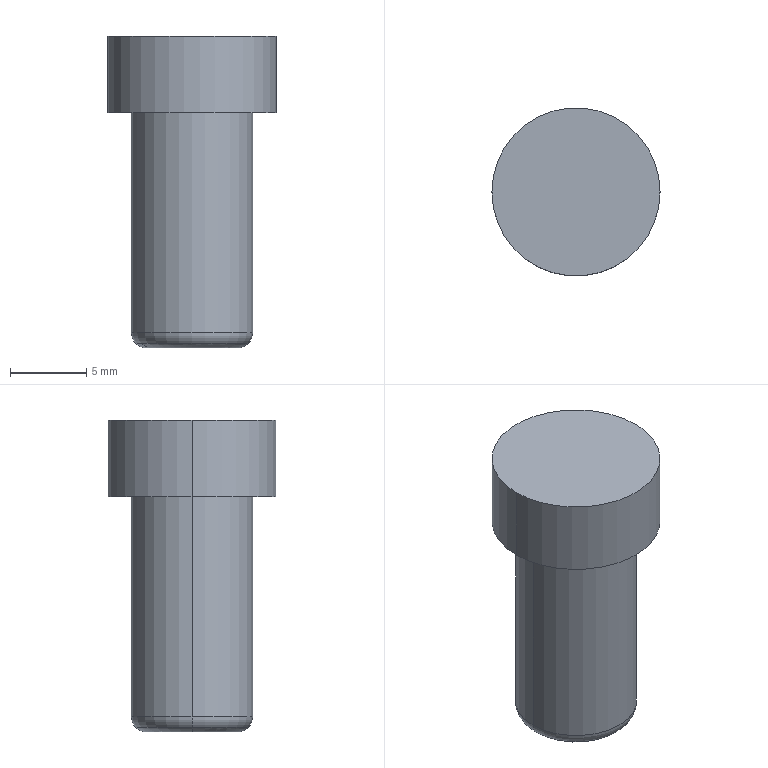Part | STEP file | 1_id1490_x_t | 1 solid | 11 faces | box 11 x 11 x 20.4 mm | volume 1232 mm3 | cylinder 4 | torus 4 | plane 3 | commonest cylinder face diameters 7.938 x2 11 x2
STEP:
#1=CARTESIAN_POINT('',(0.,0.,0.));
#2=DIRECTION('',(0.,0.,1.));
#3=DIRECTION('',(1.,0.,0.));
#4=AXIS2_PLACEMENT_3D('',#1,#2,#3);
#5=CARTESIAN_POINT('',(199.65,177.5,23.335));
#6=VERTEX_POINT('',#5);
#7=CARTESIAN_POINT('',(199.65,177.5,18.335));
#8=VERTEX_POINT('',#7);
#9=CARTESIAN_POINT('',(199.65,177.5,23.335));
#10=DIRECTION('',(0.,0.,-1.));
#11=VECTOR('',#10,1.);
#12=LINE('',#9,#11);
#13=CARTESIAN_POINT('',(194.15,177.5,23.335));
#14=DIRECTION('',(0.,0.,-1.));
#15=DIRECTION('',(-1.,0.,0.));
#16=AXIS2_PLACEMENT_3D('',#13,#14,#15);
#17=CYLINDRICAL_SURFACE('',#16,5.5);
#18=CARTESIAN_POINT('',(3.142,0.));
#19=DIRECTION('',(0.,1.));
#20=VECTOR('',#19,1.);
#21=LINE('',#18,#20);
#22=(GEOMETRIC_REPRESENTATION_CONTEXT(2)PARAMETRIC_REPRESENTATION_CONTEXT()REPRESENTATION_CONTEXT('',''));
#23=DEFINITIONAL_REPRESENTATION('',(#21),#22);
#24=PCURVE('',#17,#23);
#25=CARTESIAN_POINT('',(194.15,177.5,23.335));
#26=DIRECTION('',(0.,0.,-1.));
#27=DIRECTION('',(-1.,0.,0.));
#28=AXIS2_PLACEMENT_3D('',#25,#26,#27);
#29=CYLINDRICAL_SURFACE('',#28,5.5);
#30=CARTESIAN_POINT('',(3.142,0.));
#31=DIRECTION('',(0.,1.));
#32=VECTOR('',#31,1.);
#33=LINE('',#30,#32);
#34=(GEOMETRIC_REPRESENTATION_CONTEXT(2)PARAMETRIC_REPRESENTATION_CONTEXT()REPRESENTATION_CONTEXT('',''));
#35=DEFINITIONAL_REPRESENTATION('',(#33),#34);
#36=PCURVE('',#29,#35);
#37=SURFACE_CURVE('',#12,(#24,#36),.PCURVE_S1.);
#38=EDGE_CURVE('',#6,#8,#37,.T.);
#39=ORIENTED_EDGE('',*,*,#38,.F.);
#40=CARTESIAN_POINT('',(188.65,177.5,23.335));
#41=VERTEX_POINT('',#40);
#42=CARTESIAN_POINT('',(194.15,177.5,23.335));
#43=DIRECTION('',(0.,0.,1.));
#44=DIRECTION('',(-1.,0.,0.));
#45=AXIS2_PLACEMENT_3D('',#42,#43,#44);
#46=CIRCLE('',#45,5.5);
#47=CARTESIAN_POINT('',(6.283,0.));
#48=DIRECTION('',(-1.,0.));
#49=VECTOR('',#48,1.);
#50=LINE('',#47,#49);
#51=(GEOMETRIC_REPRESENTATION_CONTEXT(2)PARAMETRIC_REPRESENTATION_CONTEXT()REPRESENTATION_CONTEXT('',''));
#52=DEFINITIONAL_REPRESENTATION('',(#50),#51);
#53=PCURVE('',#17,#52);
#54=CARTESIAN_POINT('',(194.15,177.5,23.335));
#55=DIRECTION('',(0.,0.,1.));
#56=DIRECTION('',(1.,0.,0.));
#57=AXIS2_PLACEMENT_3D('',#54,#55,#56);
#58=PLANE('',#57);
#59=CARTESIAN_POINT('',(0.,0.));
#60=DIRECTION('',(-1.,0.));
#61=AXIS2_PLACEMENT_2D('',#59,#60);
#62=CIRCLE('',#61,5.5);
#63=(GEOMETRIC_REPRESENTATION_CONTEXT(2)PARAMETRIC_REPRESENTATION_CONTEXT()REPRESENTATION_CONTEXT('',''));
#64=DEFINITIONAL_REPRESENTATION('',(#62),#63);
#65=PCURVE('',#58,#64);
#66=SURFACE_CURVE('',#46,(#53,#65),.PCURVE_S1.);
#67=EDGE_CURVE('',#41,#6,#66,.T.);
#68=ORIENTED_EDGE('',*,*,#67,.F.);
#69=CARTESIAN_POINT('',(188.65,177.5,18.335));
#70=VERTEX_POINT('',#69);
#71=CARTESIAN_POINT('',(188.65,177.5,23.335));
#72=DIRECTION('',(0.,0.,1.));
#73=VECTOR('',#72,1.);
#74=LINE('',#71,#73);
#75=CARTESIAN_POINT('',(6.283,0.));
#76=DIRECTION('',(0.,-1.));
#77=VECTOR('',#76,1.);
#78=LINE('',#75,#77);
#79=(GEOMETRIC_REPRESENTATION_CONTEXT(2)PARAMETRIC_REPRESENTATION_CONTEXT()REPRESENTATION_CONTEXT('',''));
#80=DEFINITIONAL_REPRESENTATION('',(#78),#79);
#81=PCURVE('',#17,#80);
#82=CARTESIAN_POINT('',(0.,0.));
#83=DIRECTION('',(0.,-1.));
#84=VECTOR('',#83,1.);
#85=LINE('',#82,#84);
#86=(GEOMETRIC_REPRESENTATION_CONTEXT(2)PARAMETRIC_REPRESENTATION_CONTEXT()REPRESENTATION_CONTEXT('',''));
#87=DEFINITIONAL_REPRESENTATION('',(#85),#86);
#88=PCURVE('',#29,#87);
#89=SURFACE_CURVE('',#74,(#81,#88),.PCURVE_S1.);
#90=EDGE_CURVE('',#70,#41,#89,.T.);
#91=ORIENTED_EDGE('',*,*,#90,.F.);
#92=CARTESIAN_POINT('',(194.15,177.5,18.335));
#93=DIRECTION('',(0.,0.,-1.));
#94=DIRECTION('',(1.,0.,0.));
#95=AXIS2_PLACEMENT_3D('',#92,#93,#94);
#96=CIRCLE('',#95,5.5);
#97=CARTESIAN_POINT('',(3.142,5.));
#98=DIRECTION('',(1.,0.));
#99=VECTOR('',#98,1.);
#100=LINE('',#97,#99);
#101=(GEOMETRIC_REPRESENTATION_CONTEXT(2)PARAMETRIC_REPRESENTATION_CONTEXT()REPRESENTATION_CONTEXT('',''));
#102=DEFINITIONAL_REPRESENTATION('',(#100),#101);
#103=PCURVE('',#17,#102);
#104=CARTESIAN_POINT('',(194.15,177.5,18.335));
#105=DIRECTION('',(0.,0.,-1.));
#106=DIRECTION('',(-1.,0.,0.));
#107=AXIS2_PLACEMENT_3D('',#104,#105,#106);
#108=PLANE('',#107);
#109=CARTESIAN_POINT('',(0.,0.));
#110=DIRECTION('',(-1.,0.));
#111=AXIS2_PLACEMENT_2D('',#109,#110);
#112=CIRCLE('',#111,5.5);
#113=(GEOMETRIC_REPRESENTATION_CONTEXT(2)PARAMETRIC_REPRESENTATION_CONTEXT()REPRESENTATION_CONTEXT('',''));
#114=DEFINITIONAL_REPRESENTATION('',(#112),#113);
#115=PCURVE('',#108,#114);
#116=SURFACE_CURVE('',#96,(#103,#115),.PCURVE_S1.);
#117=EDGE_CURVE('',#8,#70,#116,.T.);
#118=ORIENTED_EDGE('',*,*,#117,.F.);
#119=EDGE_LOOP('',(#39,#68,#91,#118));
#120=FACE_BOUND('',#119,.T.);
#121=ADVANCED_FACE('',(#120),#17,.T.);
#122=ORIENTED_EDGE('',*,*,#117,.T.);
#123=CARTESIAN_POINT('',(194.15,177.5,18.335));
#124=DIRECTION('',(0.,0.,-1.));
#125=DIRECTION('',(-1.,0.,0.));
#126=AXIS2_PLACEMENT_3D('',#123,#124,#125);
#127=CIRCLE('',#126,5.5);
#128=CARTESIAN_POINT('',(0.,0.));
#129=DIRECTION('',(1.,0.));
#130=AXIS2_PLACEMENT_2D('',#128,#129);
#131=CIRCLE('',#130,5.5);
#132=(GEOMETRIC_REPRESENTATION_CONTEXT(2)PARAMETRIC_REPRESENTATION_CONTEXT()REPRESENTATION_CONTEXT('',''));
#133=DEFINITIONAL_REPRESENTATION('',(#131),#132);
#134=PCURVE('',#108,#133);
#135=CARTESIAN_POINT('',(0.,5.));
#136=DIRECTION('',(1.,0.));
#137=VECTOR('',#136,1.);
#138=LINE('',#135,#137);
#139=(GEOMETRIC_REPRESENTATION_CONTEXT(2)PARAMETRIC_REPRESENTATION_CONTEXT()REPRESENTATION_CONTEXT('',''));
#140=DEFINITIONAL_REPRESENTATION('',(#138),#139);
#141=PCURVE('',#29,#140);
#142=SURFACE_CURVE('',#127,(#134,#141),.PCURVE_S1.);
#143=EDGE_CURVE('',#70,#8,#142,.T.);
#144=ORIENTED_EDGE('',*,*,#143,.T.);
#145=EDGE_LOOP('',(#122,#144));
#146=FACE_BOUND('',#145,.T.);
#147=CARTESIAN_POINT('',(190.181,177.5,18.335));
#148=VERTEX_POINT('',#147);
#149=CARTESIAN_POINT('',(198.119,177.5,18.335));
#150=VERTEX_POINT('',#149);
#151=CARTESIAN_POINT('',(194.15,177.5,18.335));
#152=DIRECTION('',(0.,0.,1.));
#153=DIRECTION('',(-1.,0.,0.));
#154=AXIS2_PLACEMENT_3D('',#151,#152,#153);
#155=CIRCLE('',#154,3.969);
#156=CARTESIAN_POINT('',(3.969,0.));
#157=CARTESIAN_POINT('',(3.969,-6.874));
#158=CARTESIAN_POINT('',(-1.984,-3.437));
#159=CARTESIAN_POINT('',(-7.938,0.));
#160=CARTESIAN_POINT('',(-1.984,3.437));
#161=CARTESIAN_POINT('',(3.969,6.874));
#162=CARTESIAN_POINT('',(3.969,0.));
#163=(BOUNDED_CURVE()B_SPLINE_CURVE(2,(#156,#157,#158,#159,#160,#161,#162),.UNSPECIFIED.,.T.,.F.)B_SPLINE_CURVE_WITH_KNOTS((1,2,2,2,2,1),(-2.094,0.,2.094,4.189,6.283,8.378),.UNSPECIFIED.)CURVE()GEOMETRIC_REPRESENTATION_ITEM()RATIONAL_B_SPLINE_CURVE((1.,0.5,1.,0.5,1.,0.5,1.))REPRESENTATION_ITEM(''));
#164=(GEOMETRIC_REPRESENTATION_CONTEXT(2)PARAMETRIC_REPRESENTATION_CONTEXT()REPRESENTATION_CONTEXT('',''));
#165=DEFINITIONAL_REPRESENTATION('',(#163),#164);
#166=PCURVE('',#108,#165);
#167=CARTESIAN_POINT('',(194.15,177.5,23.335));
#168=DIRECTION('',(0.,0.,-1.));
#169=DIRECTION('',(-1.,0.,0.));
#170=AXIS2_PLACEMENT_3D('',#167,#168,#169);
#171=CYLINDRICAL_SURFACE('',#170,3.969);
#172=CARTESIAN_POINT('',(6.283,5.));
#173=DIRECTION('',(-1.,0.));
#174=VECTOR('',#173,1.);
#175=LINE('',#172,#174);
#176=(GEOMETRIC_REPRESENTATION_CONTEXT(2)PARAMETRIC_REPRESENTATION_CONTEXT()REPRESENTATION_CONTEXT('',''));
#177=DEFINITIONAL_REPRESENTATION('',(#175),#176);
#178=PCURVE('',#171,#177);
#179=SURFACE_CURVE('',#155,(#166,#178),.PCURVE_S1.);
#180=EDGE_CURVE('',#148,#150,#179,.T.);
#181=ORIENTED_EDGE('',*,*,#180,.T.);
#182=CARTESIAN_POINT('',(194.15,177.5,18.335));
#183=DIRECTION('',(0.,0.,1.));
#184=DIRECTION('',(1.,0.,0.));
#185=AXIS2_PLACEMENT_3D('',#182,#183,#184);
#186=CIRCLE('',#185,3.969);
#187=CARTESIAN_POINT('',(-3.969,0.));
#188=CARTESIAN_POINT('',(-3.969,6.874));
#189=CARTESIAN_POINT('',(1.984,3.437));
#190=CARTESIAN_POINT('',(7.938,0.));
#191=CARTESIAN_POINT('',(1.984,-3.437));
#192=CARTESIAN_POINT('',(-3.969,-6.874));
#193=CARTESIAN_POINT('',(-3.969,0.));
#194=(BOUNDED_CURVE()B_SPLINE_CURVE(2,(#187,#188,#189,#190,#191,#192,#193),.UNSPECIFIED.,.T.,.F.)B_SPLINE_CURVE_WITH_KNOTS((1,2,2,2,2,1),(-2.094,0.,2.094,4.189,6.283,8.378),.UNSPECIFIED.)CURVE()GEOMETRIC_REPRESENTATION_ITEM()RATIONAL_B_SPLINE_CURVE((1.,0.5,1.,0.5,1.,0.5,1.))REPRESENTATION_ITEM(''));
#195=(GEOMETRIC_REPRESENTATION_CONTEXT(2)PARAMETRIC_REPRESENTATION_CONTEXT()REPRESENTATION_CONTEXT('',''));
#196=DEFINITIONAL_REPRESENTATION('',(#194),#195);
#197=PCURVE('',#108,#196);
#198=CARTESIAN_POINT('',(194.15,177.5,23.335));
#199=DIRECTION('',(0.,0.,-1.));
#200=DIRECTION('',(-1.,0.,0.));
#201=AXIS2_PLACEMENT_3D('',#198,#199,#200);
#202=CYLINDRICAL_SURFACE('',#201,3.969);
#203=CARTESIAN_POINT('',(3.142,5.));
#204=DIRECTION('',(-1.,0.));
#205=VECTOR('',#204,1.);
#206=LINE('',#203,#205);
#207=(GEOMETRIC_REPRESENTATION_CONTEXT(2)PARAMETRIC_REPRESENTATION_CONTEXT()REPRESENTATION_CONTEXT('',''));
#208=DEFINITIONAL_REPRESENTATION('',(#206),#207);
#209=PCURVE('',#202,#208);
#210=SURFACE_CURVE('',#186,(#197,#209),.PCURVE_S1.);
#211=EDGE_CURVE('',#150,#148,#210,.T.);
#212=ORIENTED_EDGE('',*,*,#211,.T.);
#213=EDGE_LOOP('',(#181,#212));
#214=FACE_BOUND('',#213,.T.);
#215=ADVANCED_FACE('',(#146,#214),#108,.T.);
#216=CARTESIAN_POINT('',(198.119,177.5,3.935));
#217=VERTEX_POINT('',#216);
#218=CARTESIAN_POINT('',(198.119,177.5,18.335));
#219=DIRECTION('',(0.,0.,-1.));
#220=VECTOR('',#219,1.);
#221=LINE('',#218,#220);
#222=CARTESIAN_POINT('',(3.142,5.));
#223=DIRECTION('',(0.,1.));
#224=VECTOR('',#223,1.);
#225=LINE('',#222,#224);
#226=(GEOMETRIC_REPRESENTATION_CONTEXT(2)PARAMETRIC_REPRESENTATION_CONTEXT()REPRESENTATION_CONTEXT('',''));
#227=DEFINITIONAL_REPRESENTATION('',(#225),#226);
#228=PCURVE('',#202,#227);
#229=CARTESIAN_POINT('',(3.142,5.));
#230=DIRECTION('',(0.,1.));
#231=VECTOR('',#230,1.);
#232=LINE('',#229,#231);
#233=(GEOMETRIC_REPRESENTATION_CONTEXT(2)PARAMETRIC_REPRESENTATION_CONTEXT()REPRESENTATION_CONTEXT('',''));
#234=DEFINITIONAL_REPRESENTATION('',(#232),#233);
#235=PCURVE('',#171,#234);
#236=SURFACE_CURVE('',#221,(#228,#235),.PCURVE_S1.);
#237=EDGE_CURVE('',#150,#217,#236,.T.);
#238=ORIENTED_EDGE('',*,*,#237,.T.);
#239=CARTESIAN_POINT('',(190.181,177.5,3.935));
#240=VERTEX_POINT('',#239);
#241=CARTESIAN_POINT('',(194.15,177.5,3.935));
#242=DIRECTION('',(0.,0.,-1.));
#243=DIRECTION('',(-1.,0.,0.));
#244=AXIS2_PLACEMENT_3D('',#241,#242,#243);
#245=CIRCLE('',#244,3.969);
#246=CARTESIAN_POINT('',(0.,19.4));
#247=DIRECTION('',(1.,0.));
#248=VECTOR('',#247,1.);
#249=LINE('',#246,#248);
#250=(GEOMETRIC_REPRESENTATION_CONTEXT(2)PARAMETRIC_REPRESENTATION_CONTEXT()REPRESENTATION_CONTEXT('',''));
#251=DEFINITIONAL_REPRESENTATION('',(#249),#250);
#252=PCURVE('',#202,#251);
#253=CARTESIAN_POINT('',(194.15,177.5,3.935));
#254=DIRECTION('',(0.,0.,-1.));
#255=DIRECTION('',(-1.,0.,0.));
#256=AXIS2_PLACEMENT_3D('',#253,#254,#255);
#257=TOROIDAL_SURFACE('',#256,2.969,1.);
#258=CARTESIAN_POINT('',(0.,0.));
#259=DIRECTION('',(1.,0.));
#260=VECTOR('',#259,1.);
#261=LINE('',#258,#260);
#262=(GEOMETRIC_REPRESENTATION_CONTEXT(2)PARAMETRIC_REPRESENTATION_CONTEXT()REPRESENTATION_CONTEXT('',''));
#263=DEFINITIONAL_REPRESENTATION('',(#261),#262);
#264=PCURVE('',#257,#263);
#265=SURFACE_CURVE('',#245,(#252,#264),.PCURVE_S1.);
#266=EDGE_CURVE('',#240,#217,#265,.T.);
#267=ORIENTED_EDGE('',*,*,#266,.F.);
#268=CARTESIAN_POINT('',(190.181,177.5,18.335));
#269=DIRECTION('',(0.,0.,1.));
#270=VECTOR('',#269,1.);
#271=LINE('',#268,#270);
#272=CARTESIAN_POINT('',(0.,5.));
#273=DIRECTION('',(0.,-1.));
#274=VECTOR('',#273,1.);
#275=LINE('',#272,#274);
#276=(GEOMETRIC_REPRESENTATION_CONTEXT(2)PARAMETRIC_REPRESENTATION_CONTEXT()REPRESENTATION_CONTEXT('',''));
#277=DEFINITIONAL_REPRESENTATION('',(#275),#276);
#278=PCURVE('',#202,#277);
#279=CARTESIAN_POINT('',(6.283,5.));
#280=DIRECTION('',(0.,-1.));
#281=VECTOR('',#280,1.);
#282=LINE('',#279,#281);
#283=(GEOMETRIC_REPRESENTATION_CONTEXT(2)PARAMETRIC_REPRESENTATION_CONTEXT()REPRESENTATION_CONTEXT('',''));
#284=DEFINITIONAL_REPRESENTATION('',(#282),#283);
#285=PCURVE('',#171,#284);
#286=SURFACE_CURVE('',#271,(#278,#285),.PCURVE_S1.);
#287=EDGE_CURVE('',#240,#148,#286,.T.);
#288=ORIENTED_EDGE('',*,*,#287,.T.);
#289=ORIENTED_EDGE('',*,*,#211,.F.);
#290=EDGE_LOOP('',(#238,#267,#288,#289));
#291=FACE_BOUND('',#290,.T.);
#292=ADVANCED_FACE('',(#291),#202,.T.);
#293=ORIENTED_EDGE('',*,*,#287,.F.);
#294=CARTESIAN_POINT('',(194.15,177.5,3.935));
#295=DIRECTION('',(0.,0.,-1.));
#296=DIRECTION('',(1.,0.,0.));
#297=AXIS2_PLACEMENT_3D('',#294,#295,#296);
#298=CIRCLE('',#297,3.969);
#299=CARTESIAN_POINT('',(3.142,19.4));
#300=DIRECTION('',(1.,0.));
#301=VECTOR('',#300,1.);
#302=LINE('',#299,#301);
#303=(GEOMETRIC_REPRESENTATION_CONTEXT(2)PARAMETRIC_REPRESENTATION_CONTEXT()REPRESENTATION_CONTEXT('',''));
#304=DEFINITIONAL_REPRESENTATION('',(#302),#303);
#305=PCURVE('',#171,#304);
#306=CARTESIAN_POINT('',(194.15,177.5,3.935));
#307=DIRECTION('',(0.,0.,-1.));
#308=DIRECTION('',(-1.,0.,0.));
#309=AXIS2_PLACEMENT_3D('',#306,#307,#308);
#310=TOROIDAL_SURFACE('',#309,2.969,1.);
#311=CARTESIAN_POINT('',(3.142,0.));
#312=DIRECTION('',(1.,0.));
#313=VECTOR('',#312,1.);
#314=LINE('',#311,#313);
#315=(GEOMETRIC_REPRESENTATION_CONTEXT(2)PARAMETRIC_REPRESENTATION_CONTEXT()REPRESENTATION_CONTEXT('',''));
#316=DEFINITIONAL_REPRESENTATION('',(#314),#315);
#317=PCURVE('',#310,#316);
#318=SURFACE_CURVE('',#298,(#305,#317),.PCURVE_S1.);
#319=EDGE_CURVE('',#217,#240,#318,.T.);
#320=ORIENTED_EDGE('',*,*,#319,.F.);
#321=ORIENTED_EDGE('',*,*,#237,.F.);
#322=ORIENTED_EDGE('',*,*,#180,.F.);
#323=EDGE_LOOP('',(#293,#320,#321,#322));
#324=FACE_BOUND('',#323,.T.);
#325=ADVANCED_FACE('',(#324),#171,.T.);
#326=CARTESIAN_POINT('',(190.474,177.5,3.228));
#327=VERTEX_POINT('',#326);
#328=CARTESIAN_POINT('',(191.181,177.5,3.935));
#329=DIRECTION('',(0.,1.,0.));
#330=DIRECTION('',(-1.,0.,0.));
#331=AXIS2_PLACEMENT_3D('',#328,#329,#330);
#332=CIRCLE('',#331,1.);
#333=CARTESIAN_POINT('',(6.283,6.283));
#334=DIRECTION('',(0.,-1.));
#335=VECTOR('',#334,1.);
#336=LINE('',#333,#335);
#337=(GEOMETRIC_REPRESENTATION_CONTEXT(2)PARAMETRIC_REPRESENTATION_CONTEXT()REPRESENTATION_CONTEXT('',''));
#338=DEFINITIONAL_REPRESENTATION('',(#336),#337);
#339=PCURVE('',#310,#338);
#340=CARTESIAN_POINT('',(0.,6.283));
#341=DIRECTION('',(0.,-1.));
#342=VECTOR('',#341,1.);
#343=LINE('',#340,#342);
#344=(GEOMETRIC_REPRESENTATION_CONTEXT(2)PARAMETRIC_REPRESENTATION_CONTEXT()REPRESENTATION_CONTEXT('',''));
#345=DEFINITIONAL_REPRESENTATION('',(#343),#344);
#346=PCURVE('',#257,#345);
#347=SURFACE_CURVE('',#332,(#339,#346),.PCURVE_S1.);
#348=EDGE_CURVE('',#327,#240,#347,.T.);
#349=ORIENTED_EDGE('',*,*,#348,.F.);
#350=CARTESIAN_POINT('',(197.826,177.5,3.228));
#351=VERTEX_POINT('',#350);
#352=CARTESIAN_POINT('',(194.15,177.5,3.228));
#353=DIRECTION('',(0.,0.,-1.));
#354=DIRECTION('',(1.,0.,0.));
#355=AXIS2_PLACEMENT_3D('',#352,#353,#354);
#356=CIRCLE('',#355,3.676);
#357=CARTESIAN_POINT('',(3.142,0.7854));
#358=DIRECTION('',(1.,0.));
#359=VECTOR('',#358,1.);
#360=LINE('',#357,#359);
#361=(GEOMETRIC_REPRESENTATION_CONTEXT(2)PARAMETRIC_REPRESENTATION_CONTEXT()REPRESENTATION_CONTEXT('',''));
#362=DEFINITIONAL_REPRESENTATION('',(#360),#361);
#363=PCURVE('',#310,#362);
#364=CARTESIAN_POINT('',(194.15,177.5,3.935));
#365=DIRECTION('',(0.,0.,-1.));
#366=DIRECTION('',(-1.,0.,0.));
#367=AXIS2_PLACEMENT_3D('',#364,#365,#366);
#368=TOROIDAL_SURFACE('',#367,2.969,1.);
#369=CARTESIAN_POINT('',(3.142,0.7854));
#370=DIRECTION('',(1.,0.));
#371=VECTOR('',#370,1.);
#372=LINE('',#369,#371);
#373=(GEOMETRIC_REPRESENTATION_CONTEXT(2)PARAMETRIC_REPRESENTATION_CONTEXT()REPRESENTATION_CONTEXT('',''));
#374=DEFINITIONAL_REPRESENTATION('',(#372),#373);
#375=PCURVE('',#368,#374);
#376=SURFACE_CURVE('',#356,(#363,#375),.PCURVE_S1.);
#377=EDGE_CURVE('',#351,#327,#376,.T.);
#378=ORIENTED_EDGE('',*,*,#377,.F.);
#379=CARTESIAN_POINT('',(197.119,177.5,3.935));
#380=DIRECTION('',(0.,1.,0.));
#381=DIRECTION('',(1.,0.,0.));
#382=AXIS2_PLACEMENT_3D('',#379,#380,#381);
#383=CIRCLE('',#382,1.);
#384=CARTESIAN_POINT('',(3.142,0.));
#385=DIRECTION('',(0.,1.));
#386=VECTOR('',#385,1.);
#387=LINE('',#384,#386);
#388=(GEOMETRIC_REPRESENTATION_CONTEXT(2)PARAMETRIC_REPRESENTATION_CONTEXT()REPRESENTATION_CONTEXT('',''));
#389=DEFINITIONAL_REPRESENTATION('',(#387),#388);
#390=PCURVE('',#310,#389);
#391=CARTESIAN_POINT('',(3.142,0.));
#392=DIRECTION('',(0.,1.));
#393=VECTOR('',#392,1.);
#394=LINE('',#391,#393);
#395=(GEOMETRIC_REPRESENTATION_CONTEXT(2)PARAMETRIC_REPRESENTATION_CONTEXT()REPRESENTATION_CONTEXT('',''));
#396=DEFINITIONAL_REPRESENTATION('',(#394),#395);
#397=PCURVE('',#257,#396);
#398=SURFACE_CURVE('',#383,(#390,#397),.PCURVE_S1.);
#399=EDGE_CURVE('',#217,#351,#398,.T.);
#400=ORIENTED_EDGE('',*,*,#399,.F.);
#401=ORIENTED_EDGE('',*,*,#319,.T.);
#402=EDGE_LOOP('',(#349,#378,#400,#401));
#403=FACE_BOUND('',#402,.T.);
#404=ADVANCED_FACE('',(#403),#310,.T.);
#405=ORIENTED_EDGE('',*,*,#399,.T.);
#406=CARTESIAN_POINT('',(194.15,177.5,3.228));
#407=DIRECTION('',(0.,0.,-1.));
#408=DIRECTION('',(-1.,0.,0.));
#409=AXIS2_PLACEMENT_3D('',#406,#407,#408);
#410=CIRCLE('',#409,3.676);
#411=CARTESIAN_POINT('',(0.,0.7854));
#412=DIRECTION('',(1.,0.));
#413=VECTOR('',#412,1.);
#414=LINE('',#411,#413);
#415=(GEOMETRIC_REPRESENTATION_CONTEXT(2)PARAMETRIC_REPRESENTATION_CONTEXT()REPRESENTATION_CONTEXT('',''));
#416=DEFINITIONAL_REPRESENTATION('',(#414),#415);
#417=PCURVE('',#257,#416);
#418=CARTESIAN_POINT('',(194.15,177.5,3.935));
#419=DIRECTION('',(0.,0.,-1.));
#420=DIRECTION('',(-1.,0.,0.));
#421=AXIS2_PLACEMENT_3D('',#418,#419,#420);
#422=TOROIDAL_SURFACE('',#421,2.969,1.);
#423=CARTESIAN_POINT('',(0.,0.7854));
#424=DIRECTION('',(1.,0.));
#425=VECTOR('',#424,1.);
#426=LINE('',#423,#425);
#427=(GEOMETRIC_REPRESENTATION_CONTEXT(2)PARAMETRIC_REPRESENTATION_CONTEXT()REPRESENTATION_CONTEXT('',''));
#428=DEFINITIONAL_REPRESENTATION('',(#426),#427);
#429=PCURVE('',#422,#428);
#430=SURFACE_CURVE('',#410,(#417,#429),.PCURVE_S1.);
#431=EDGE_CURVE('',#327,#351,#430,.T.);
#432=ORIENTED_EDGE('',*,*,#431,.F.);
#433=ORIENTED_EDGE('',*,*,#348,.T.);
#434=ORIENTED_EDGE('',*,*,#266,.T.);
#435=EDGE_LOOP('',(#405,#432,#433,#434));
#436=FACE_BOUND('',#435,.T.);
#437=ADVANCED_FACE('',(#436),#257,.T.);
#438=CARTESIAN_POINT('',(191.181,177.5,2.935));
#439=VERTEX_POINT('',#438);
#440=CARTESIAN_POINT('',(191.181,177.5,3.935));
#441=DIRECTION('',(0.,-1.,0.));
#442=DIRECTION('',(-0.7071,0.,-0.7071));
#443=AXIS2_PLACEMENT_3D('',#440,#441,#442);
#444=CIRCLE('',#443,1.);
#445=CARTESIAN_POINT('',(0.,0.7854));
#446=DIRECTION('',(0.,1.));
#447=VECTOR('',#446,1.);
#448=LINE('',#445,#447);
#449=(GEOMETRIC_REPRESENTATION_CONTEXT(2)PARAMETRIC_REPRESENTATION_CONTEXT()REPRESENTATION_CONTEXT('',''));
#450=DEFINITIONAL_REPRESENTATION('',(#448),#449);
#451=PCURVE('',#422,#450);
#452=CARTESIAN_POINT('',(6.283,0.7854));
#453=DIRECTION('',(0.,1.));
#454=VECTOR('',#453,1.);
#455=LINE('',#452,#454);
#456=(GEOMETRIC_REPRESENTATION_CONTEXT(2)PARAMETRIC_REPRESENTATION_CONTEXT()REPRESENTATION_CONTEXT('',''));
#457=DEFINITIONAL_REPRESENTATION('',(#455),#456);
#458=PCURVE('',#368,#457);
#459=SURFACE_CURVE('',#444,(#451,#458),.PCURVE_S1.);
#460=EDGE_CURVE('',#327,#439,#459,.T.);
#461=ORIENTED_EDGE('',*,*,#460,.F.);
#462=ORIENTED_EDGE('',*,*,#431,.T.);
#463=CARTESIAN_POINT('',(197.119,177.5,2.935));
#464=VERTEX_POINT('',#463);
#465=CARTESIAN_POINT('',(197.119,177.5,3.935));
#466=DIRECTION('',(0.,-1.,0.));
#467=DIRECTION('',(0.7071,0.,-0.7071));
#468=AXIS2_PLACEMENT_3D('',#465,#466,#467);
#469=CIRCLE('',#468,1.);
#470=CARTESIAN_POINT('',(3.142,7.069));
#471=DIRECTION('',(0.,-1.));
#472=VECTOR('',#471,1.);
#473=LINE('',#470,#472);
#474=(GEOMETRIC_REPRESENTATION_CONTEXT(2)PARAMETRIC_REPRESENTATION_CONTEXT()REPRESENTATION_CONTEXT('',''));
#475=DEFINITIONAL_REPRESENTATION('',(#473),#474);
#476=PCURVE('',#422,#475);
#477=CARTESIAN_POINT('',(3.142,7.069));
#478=DIRECTION('',(0.,-1.));
#479=VECTOR('',#478,1.);
#480=LINE('',#477,#479);
#481=(GEOMETRIC_REPRESENTATION_CONTEXT(2)PARAMETRIC_REPRESENTATION_CONTEXT()REPRESENTATION_CONTEXT('',''));
#482=DEFINITIONAL_REPRESENTATION('',(#480),#481);
#483=PCURVE('',#368,#482);
#484=SURFACE_CURVE('',#469,(#476,#483),.PCURVE_S1.);
#485=EDGE_CURVE('',#464,#351,#484,.T.);
#486=ORIENTED_EDGE('',*,*,#485,.F.);
#487=CARTESIAN_POINT('',(194.15,177.5,2.935));
#488=DIRECTION('',(0.,0.,-1.));
#489=DIRECTION('',(-1.,0.,0.));
#490=AXIS2_PLACEMENT_3D('',#487,#488,#489);
#491=CIRCLE('',#490,2.969);
#492=CARTESIAN_POINT('',(0.,1.571));
#493=DIRECTION('',(1.,0.));
#494=VECTOR('',#493,1.);
#495=LINE('',#492,#494);
#496=(GEOMETRIC_REPRESENTATION_CONTEXT(2)PARAMETRIC_REPRESENTATION_CONTEXT()REPRESENTATION_CONTEXT('',''));
#497=DEFINITIONAL_REPRESENTATION('',(#495),#496);
#498=PCURVE('',#422,#497);
#499=CARTESIAN_POINT('',(194.15,177.5,2.935));
#500=DIRECTION('',(0.,0.,-1.));
#501=DIRECTION('',(-1.,0.,0.));
#502=AXIS2_PLACEMENT_3D('',#499,#500,#501);
#503=PLANE('',#502);
#504=CARTESIAN_POINT('',(0.,0.));
#505=DIRECTION('',(1.,0.));
#506=AXIS2_PLACEMENT_2D('',#504,#505);
#507=CIRCLE('',#506,2.969);
#508=(GEOMETRIC_REPRESENTATION_CONTEXT(2)PARAMETRIC_REPRESENTATION_CONTEXT()REPRESENTATION_CONTEXT('',''));
#509=DEFINITIONAL_REPRESENTATION('',(#507),#508);
#510=PCURVE('',#503,#509);
#511=SURFACE_CURVE('',#491,(#498,#510),.PCURVE_S1.);
#512=EDGE_CURVE('',#439,#464,#511,.T.);
#513=ORIENTED_EDGE('',*,*,#512,.F.);
#514=EDGE_LOOP('',(#461,#462,#486,#513));
#515=FACE_BOUND('',#514,.T.);
#516=ADVANCED_FACE('',(#515),#422,.T.);
#517=ORIENTED_EDGE('',*,*,#512,.T.);
#518=CARTESIAN_POINT('',(194.15,177.5,2.935));
#519=DIRECTION('',(0.,0.,-1.));
#520=DIRECTION('',(1.,0.,0.));
#521=AXIS2_PLACEMENT_3D('',#518,#519,#520);
#522=CIRCLE('',#521,2.969);
#523=CARTESIAN_POINT('',(0.,0.));
#524=DIRECTION('',(-1.,0.));
#525=AXIS2_PLACEMENT_2D('',#523,#524);
#526=CIRCLE('',#525,2.969);
#527=(GEOMETRIC_REPRESENTATION_CONTEXT(2)PARAMETRIC_REPRESENTATION_CONTEXT()REPRESENTATION_CONTEXT('',''));
#528=DEFINITIONAL_REPRESENTATION('',(#526),#527);
#529=PCURVE('',#503,#528);
#530=CARTESIAN_POINT('',(3.142,1.571));
#531=DIRECTION('',(1.,0.));
#532=VECTOR('',#531,1.);
#533=LINE('',#530,#532);
#534=(GEOMETRIC_REPRESENTATION_CONTEXT(2)PARAMETRIC_REPRESENTATION_CONTEXT()REPRESENTATION_CONTEXT('',''));
#535=DEFINITIONAL_REPRESENTATION('',(#533),#534);
#536=PCURVE('',#368,#535);
#537=SURFACE_CURVE('',#522,(#529,#536),.PCURVE_S1.);
#538=EDGE_CURVE('',#464,#439,#537,.T.);
#539=ORIENTED_EDGE('',*,*,#538,.T.);
#540=EDGE_LOOP('',(#517,#539));
#541=FACE_BOUND('',#540,.T.);
#542=ADVANCED_FACE('',(#541),#503,.T.);
#543=ORIENTED_EDGE('',*,*,#485,.T.);
#544=ORIENTED_EDGE('',*,*,#377,.T.);
#545=ORIENTED_EDGE('',*,*,#460,.T.);
#546=ORIENTED_EDGE('',*,*,#538,.F.);
#547=EDGE_LOOP('',(#543,#544,#545,#546));
#548=FACE_BOUND('',#547,.T.);
#549=ADVANCED_FACE('',(#548),#368,.T.);
#550=ORIENTED_EDGE('',*,*,#90,.T.);
#551=CARTESIAN_POINT('',(194.15,177.5,23.335));
#552=DIRECTION('',(0.,0.,1.));
#553=DIRECTION('',(1.,0.,0.));
#554=AXIS2_PLACEMENT_3D('',#551,#552,#553);
#555=CIRCLE('',#554,5.5);
#556=CARTESIAN_POINT('',(3.142,0.));
#557=DIRECTION('',(-1.,0.));
#558=VECTOR('',#557,1.);
#559=LINE('',#556,#558);
#560=(GEOMETRIC_REPRESENTATION_CONTEXT(2)PARAMETRIC_REPRESENTATION_CONTEXT()REPRESENTATION_CONTEXT('',''));
#561=DEFINITIONAL_REPRESENTATION('',(#559),#560);
#562=PCURVE('',#29,#561);
#563=CARTESIAN_POINT('',(0.,0.));
#564=DIRECTION('',(1.,0.));
#565=AXIS2_PLACEMENT_2D('',#563,#564);
#566=CIRCLE('',#565,5.5);
#567=(GEOMETRIC_REPRESENTATION_CONTEXT(2)PARAMETRIC_REPRESENTATION_CONTEXT()REPRESENTATION_CONTEXT('',''));
#568=DEFINITIONAL_REPRESENTATION('',(#566),#567);
#569=PCURVE('',#58,#568);
#570=SURFACE_CURVE('',#555,(#562,#569),.PCURVE_S1.);
#571=EDGE_CURVE('',#6,#41,#570,.T.);
#572=ORIENTED_EDGE('',*,*,#571,.F.);
#573=ORIENTED_EDGE('',*,*,#38,.T.);
#574=ORIENTED_EDGE('',*,*,#143,.F.);
#575=EDGE_LOOP('',(#550,#572,#573,#574));
#576=FACE_BOUND('',#575,.T.);
#577=ADVANCED_FACE('',(#576),#29,.T.);
#578=ORIENTED_EDGE('',*,*,#67,.T.);
#579=ORIENTED_EDGE('',*,*,#571,.T.);
#580=EDGE_LOOP('',(#578,#579));
#581=FACE_BOUND('',#580,.T.);
#582=ADVANCED_FACE('',(#581),#58,.T.);
#583=CLOSED_SHELL('',(#121,#215,#292,#325,#404,#437,#516,#542,#549,#577,#582));
#584=MANIFOLD_SOLID_BREP('',#583);
#585=(LENGTH_UNIT()NAMED_UNIT(*)SI_UNIT(.MILLI.,.METRE.));
#586=UNCERTAINTY_MEASURE_WITH_UNIT(LENGTH_MEASURE(0.0000001),#585,'','');
#587=(NAMED_UNIT(*)PLANE_ANGLE_UNIT()SI_UNIT($,.RADIAN.));
#588=(NAMED_UNIT(*)SI_UNIT($,.STERADIAN.)SOLID_ANGLE_UNIT());
#589=(GEOMETRIC_REPRESENTATION_CONTEXT(3)GLOBAL_UNCERTAINTY_ASSIGNED_CONTEXT((#586))GLOBAL_UNIT_ASSIGNED_CONTEXT((#585,#587,#588))REPRESENTATION_CONTEXT('',''));
#590=ADVANCED_BREP_SHAPE_REPRESENTATION('',(#4,#584),#589);